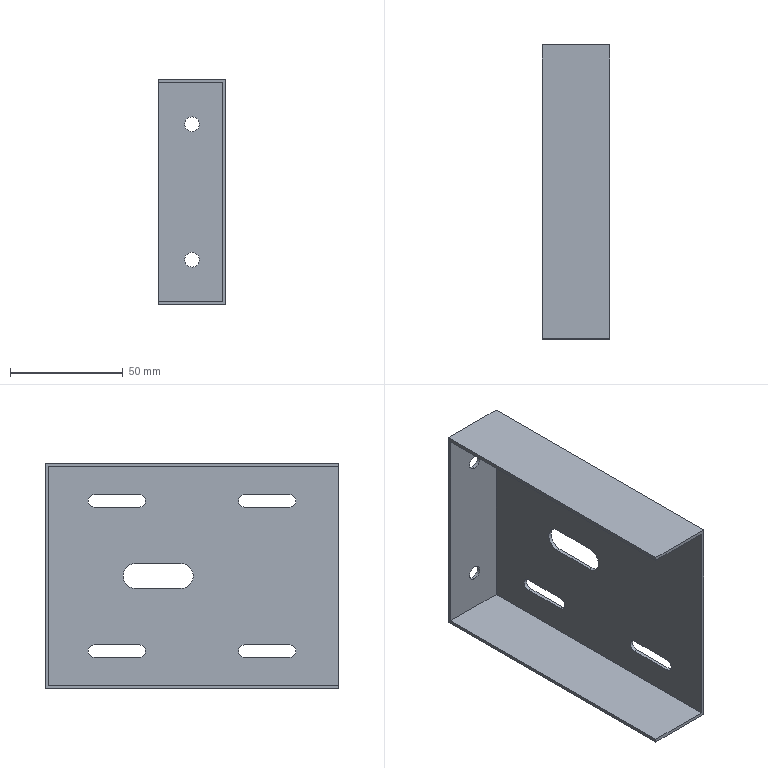Part | STEP file | 02-10 Motor fixing plate | 1 solid | 34 faces | box 30 x 130 x 100 mm | volume 33387 mm3 | plane 20 | cylinder 14 | commonest cylinder face diameters 5.5 x8 6.5 x4 11 x2